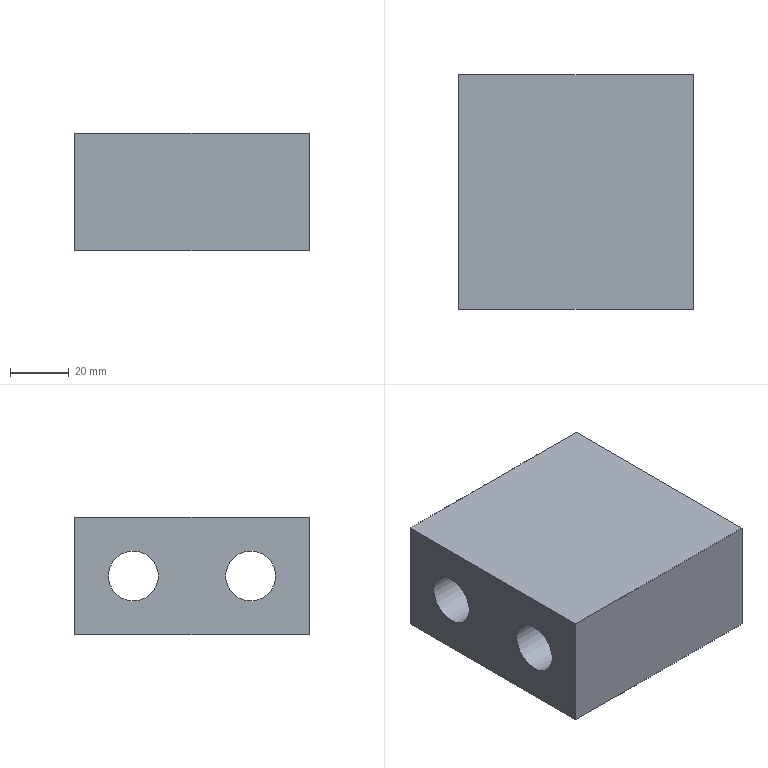Part | STEP file | 1 solid | 12 faces | box 80 x 80 x 40 mm | volume 195367 mm3 | plane 8 | cylinder 4 | commonest cylinder face diameters 17 x2 26 x2
STEP:
#1=CARTESIAN_POINT('',(350.,-102.5,-147.));
#2=VERTEX_POINT('',#1);
#3=CARTESIAN_POINT('',(350.,-102.5,-107.));
#4=VERTEX_POINT('',#3);
#5=CARTESIAN_POINT('',(350.,-102.5,-107.));
#6=DIRECTION('',(0.,0.,1.));
#7=VECTOR('',#6,1.);
#8=LINE('',#5,#7);
#9=EDGE_CURVE('',#2,#4,#8,.T.);
#10=ORIENTED_EDGE('',*,*,#9,.T.);
#11=CARTESIAN_POINT('',(430.,-102.5,-107.));
#12=VERTEX_POINT('',#11);
#13=CARTESIAN_POINT('',(350.,-102.5,-107.));
#14=DIRECTION('',(-1.,0.,0.));
#15=VECTOR('',#14,1.);
#16=LINE('',#13,#15);
#17=EDGE_CURVE('',#12,#4,#16,.T.);
#18=ORIENTED_EDGE('',*,*,#17,.F.);
#19=CARTESIAN_POINT('',(430.,-102.5,-147.));
#20=VERTEX_POINT('',#19);
#21=CARTESIAN_POINT('',(430.,-102.5,-107.));
#22=DIRECTION('',(0.,0.,1.));
#23=VECTOR('',#22,1.);
#24=LINE('',#21,#23);
#25=EDGE_CURVE('',#20,#12,#24,.T.);
#26=ORIENTED_EDGE('',*,*,#25,.F.);
#27=CARTESIAN_POINT('',(390.,-102.5,-147.));
#28=DIRECTION('',(1.,0.,0.));
#29=VECTOR('',#28,1.);
#30=LINE('',#27,#29);
#31=EDGE_CURVE('',#2,#20,#30,.T.);
#32=ORIENTED_EDGE('',*,*,#31,.F.);
#33=EDGE_LOOP('',(#10,#18,#26,#32));
#34=FACE_OUTER_BOUND('',#33,.T.);
#35=CARTESIAN_POINT('',(390.,-102.5,-127.));
#36=DIRECTION('',(0.,1.,0.));
#37=DIRECTION('',(0.,0.,1.));
#38=AXIS2_PLACEMENT_3D('',#35,#36,#37);
#39=PLANE('',#38);
#40=ADVANCED_FACE('',(#34),#39,.T.);
#41=CARTESIAN_POINT('',(350.,-182.5,-147.));
#42=VERTEX_POINT('',#41);
#43=CARTESIAN_POINT('',(430.,-182.5,-147.));
#44=VERTEX_POINT('',#43);
#45=CARTESIAN_POINT('',(350.,-182.5,-147.));
#46=DIRECTION('',(1.,0.,0.));
#47=VECTOR('',#46,1.);
#48=LINE('',#45,#47);
#49=EDGE_CURVE('',#42,#44,#48,.T.);
#50=ORIENTED_EDGE('',*,*,#49,.T.);
#51=CARTESIAN_POINT('',(430.,-182.5,-107.));
#52=VERTEX_POINT('',#51);
#53=CARTESIAN_POINT('',(430.,-182.5,-107.));
#54=DIRECTION('',(0.,0.,1.));
#55=VECTOR('',#54,1.);
#56=LINE('',#53,#55);
#57=EDGE_CURVE('',#44,#52,#56,.T.);
#58=ORIENTED_EDGE('',*,*,#57,.T.);
#59=CARTESIAN_POINT('',(350.,-182.5,-107.));
#60=VERTEX_POINT('',#59);
#61=CARTESIAN_POINT('',(350.,-182.5,-107.));
#62=DIRECTION('',(-1.,0.,0.));
#63=VECTOR('',#62,1.);
#64=LINE('',#61,#63);
#65=EDGE_CURVE('',#52,#60,#64,.T.);
#66=ORIENTED_EDGE('',*,*,#65,.T.);
#67=CARTESIAN_POINT('',(350.,-182.5,-107.));
#68=DIRECTION('',(0.,0.,1.));
#69=VECTOR('',#68,1.);
#70=LINE('',#67,#69);
#71=EDGE_CURVE('',#42,#60,#70,.T.);
#72=ORIENTED_EDGE('',*,*,#71,.F.);
#73=EDGE_LOOP('',(#50,#58,#66,#72));
#74=FACE_OUTER_BOUND('',#73,.T.);
#75=CARTESIAN_POINT('',(350.,-182.5,-107.));
#76=DIRECTION('',(0.,-1.,0.));
#77=DIRECTION('',(0.,0.,-1.));
#78=AXIS2_PLACEMENT_3D('',#75,#76,#77);
#79=PLANE('',#78);
#80=ADVANCED_FACE('',(#74),#79,.T.);
#81=CARTESIAN_POINT('',(350.,109.,-147.));
#82=DIRECTION('',(0.,-1.,0.));
#83=VECTOR('',#82,1.);
#84=LINE('',#81,#83);
#85=EDGE_CURVE('',#2,#42,#84,.T.);
#86=ORIENTED_EDGE('',*,*,#85,.F.);
#87=ORIENTED_EDGE('',*,*,#31,.T.);
#88=CARTESIAN_POINT('',(430.,109.,-147.));
#89=DIRECTION('',(0.,1.,0.));
#90=VECTOR('',#89,1.);
#91=LINE('',#88,#90);
#92=EDGE_CURVE('',#44,#20,#91,.T.);
#93=ORIENTED_EDGE('',*,*,#92,.F.);
#94=ORIENTED_EDGE('',*,*,#49,.F.);
#95=EDGE_LOOP('',(#86,#87,#93,#94));
#96=FACE_OUTER_BOUND('',#95,.T.);
#97=CARTESIAN_POINT('',(390.,110.,-147.));
#98=DIRECTION('',(0.,0.,-1.));
#99=DIRECTION('',(-1.,0.,0.));
#100=AXIS2_PLACEMENT_3D('',#97,#98,#99);
#101=PLANE('',#100);
#102=ADVANCED_FACE('',(#96),#101,.T.);
#103=ORIENTED_EDGE('',*,*,#17,.T.);
#104=CARTESIAN_POINT('',(350.,109.,-107.));
#105=DIRECTION('',(0.,-1.,0.));
#106=VECTOR('',#105,1.);
#107=LINE('',#104,#106);
#108=EDGE_CURVE('',#4,#60,#107,.T.);
#109=ORIENTED_EDGE('',*,*,#108,.T.);
#110=ORIENTED_EDGE('',*,*,#65,.F.);
#111=CARTESIAN_POINT('',(430.,109.,-107.));
#112=DIRECTION('',(0.,-1.,0.));
#113=VECTOR('',#112,1.);
#114=LINE('',#111,#113);
#115=EDGE_CURVE('',#12,#52,#114,.T.);
#116=ORIENTED_EDGE('',*,*,#115,.F.);
#117=EDGE_LOOP('',(#103,#109,#110,#116));
#118=FACE_OUTER_BOUND('',#117,.T.);
#119=CARTESIAN_POINT('',(350.,109.,-107.));
#120=DIRECTION('',(0.,0.,1.));
#121=DIRECTION('',(0.,-1.,0.));
#122=AXIS2_PLACEMENT_3D('',#119,#120,#121);
#123=PLANE('',#122);
#124=ADVANCED_FACE('',(#118),#123,.T.);
#125=CARTESIAN_POINT('',(430.,-122.5,-140.));
#126=VERTEX_POINT('',#125);
#127=CARTESIAN_POINT('',(430.,-122.5,-127.));
#128=DIRECTION('',(1.,0.,0.));
#129=DIRECTION('',(0.,0.,-1.));
#130=AXIS2_PLACEMENT_3D('',#127,#128,#129);
#131=CIRCLE('',#130,13.);
#132=EDGE_CURVE('',#126,#126,#131,.T.);
#133=ORIENTED_EDGE('',*,*,#132,.F.);
#134=EDGE_LOOP('',(#133));
#135=FACE_BOUND('',#134,.T.);
#136=CARTESIAN_POINT('',(430.,-162.5,-140.));
#137=VERTEX_POINT('',#136);
#138=CARTESIAN_POINT('',(430.,-162.5,-127.));
#139=DIRECTION('',(-1.,0.,0.));
#140=DIRECTION('',(0.,0.,-1.));
#141=AXIS2_PLACEMENT_3D('',#138,#139,#140);
#142=CIRCLE('',#141,13.);
#143=EDGE_CURVE('',#137,#137,#142,.T.);
#144=ORIENTED_EDGE('',*,*,#143,.T.);
#145=EDGE_LOOP('',(#144));
#146=FACE_BOUND('',#145,.T.);
#147=ORIENTED_EDGE('',*,*,#25,.T.);
#148=ORIENTED_EDGE('',*,*,#115,.T.);
#149=ORIENTED_EDGE('',*,*,#57,.F.);
#150=ORIENTED_EDGE('',*,*,#92,.T.);
#151=EDGE_LOOP('',(#147,#148,#149,#150));
#152=FACE_BOUND('',#151,.T.);
#153=CARTESIAN_POINT('',(430.,109.,-107.));
#154=DIRECTION('',(1.,0.,0.));
#155=DIRECTION('',(0.,-1.,0.));
#156=AXIS2_PLACEMENT_3D('',#153,#154,#155);
#157=PLANE('',#156);
#158=ADVANCED_FACE('',(#135,#146,#152),#157,.T.);
#159=CARTESIAN_POINT('',(350.,-122.5,-135.5));
#160=VERTEX_POINT('',#159);
#161=CARTESIAN_POINT('',(350.,-122.5,-127.));
#162=DIRECTION('',(-1.,0.,0.));
#163=DIRECTION('',(0.,0.,-1.));
#164=AXIS2_PLACEMENT_3D('',#161,#162,#163);
#165=CIRCLE('',#164,8.5);
#166=EDGE_CURVE('',#160,#160,#165,.T.);
#167=ORIENTED_EDGE('',*,*,#166,.F.);
#168=EDGE_LOOP('',(#167));
#169=FACE_BOUND('',#168,.T.);
#170=CARTESIAN_POINT('',(350.,-162.5,-135.5));
#171=VERTEX_POINT('',#170);
#172=CARTESIAN_POINT('',(350.,-162.5,-127.));
#173=DIRECTION('',(1.,0.,0.));
#174=DIRECTION('',(0.,0.,-1.));
#175=AXIS2_PLACEMENT_3D('',#172,#173,#174);
#176=CIRCLE('',#175,8.5);
#177=EDGE_CURVE('',#171,#171,#176,.T.);
#178=ORIENTED_EDGE('',*,*,#177,.T.);
#179=EDGE_LOOP('',(#178));
#180=FACE_BOUND('',#179,.T.);
#181=ORIENTED_EDGE('',*,*,#108,.F.);
#182=ORIENTED_EDGE('',*,*,#9,.F.);
#183=ORIENTED_EDGE('',*,*,#85,.T.);
#184=ORIENTED_EDGE('',*,*,#71,.T.);
#185=EDGE_LOOP('',(#181,#182,#183,#184));
#186=FACE_BOUND('',#185,.T.);
#187=CARTESIAN_POINT('',(350.,109.,-107.));
#188=DIRECTION('',(1.,0.,0.));
#189=DIRECTION('',(0.,-1.,0.));
#190=AXIS2_PLACEMENT_3D('',#187,#188,#189);
#191=PLANE('',#190);
#192=ADVANCED_FACE('',(#169,#180,#186),#191,.F.);
#193=CARTESIAN_POINT('',(390.,-162.5,-118.5));
#194=VERTEX_POINT('',#193);
#195=CARTESIAN_POINT('',(390.,-162.5,-127.));
#196=DIRECTION('',(-1.,0.,0.));
#197=DIRECTION('',(0.,0.,1.));
#198=AXIS2_PLACEMENT_3D('',#195,#196,#197);
#199=CIRCLE('',#198,8.5);
#200=EDGE_CURVE('',#194,#194,#199,.T.);
#201=ORIENTED_EDGE('',*,*,#200,.F.);
#202=EDGE_LOOP('',(#201));
#203=FACE_BOUND('',#202,.T.);
#204=ORIENTED_EDGE('',*,*,#177,.F.);
#205=EDGE_LOOP('',(#204));
#206=FACE_BOUND('',#205,.T.);
#207=CARTESIAN_POINT('',(350.,-162.5,-127.));
#208=DIRECTION('',(1.,0.,0.));
#209=DIRECTION('',(0.,0.,-1.));
#210=AXIS2_PLACEMENT_3D('',#207,#208,#209);
#211=CYLINDRICAL_SURFACE('',#210,8.5);
#212=ADVANCED_FACE('',(#203,#206),#211,.F.);
#213=ORIENTED_EDGE('',*,*,#200,.T.);
#214=EDGE_LOOP('',(#213));
#215=FACE_BOUND('',#214,.T.);
#216=CARTESIAN_POINT('',(390.,-162.5,-140.));
#217=VERTEX_POINT('',#216);
#218=CARTESIAN_POINT('',(390.,-162.5,-127.));
#219=DIRECTION('',(-1.,0.,0.));
#220=DIRECTION('',(0.,0.,-1.));
#221=AXIS2_PLACEMENT_3D('',#218,#219,#220);
#222=CIRCLE('',#221,13.);
#223=EDGE_CURVE('',#217,#217,#222,.T.);
#224=ORIENTED_EDGE('',*,*,#223,.F.);
#225=EDGE_LOOP('',(#224));
#226=FACE_BOUND('',#225,.T.);
#227=CARTESIAN_POINT('',(390.,-162.5,-127.));
#228=DIRECTION('',(-1.,0.,0.));
#229=DIRECTION('',(0.,0.,1.));
#230=AXIS2_PLACEMENT_3D('',#227,#228,#229);
#231=PLANE('',#230);
#232=ADVANCED_FACE('',(#215,#226),#231,.F.);
#233=ORIENTED_EDGE('',*,*,#143,.F.);
#234=EDGE_LOOP('',(#233));
#235=FACE_BOUND('',#234,.T.);
#236=ORIENTED_EDGE('',*,*,#223,.T.);
#237=EDGE_LOOP('',(#236));
#238=FACE_BOUND('',#237,.T.);
#239=CARTESIAN_POINT('',(390.,-162.5,-127.));
#240=DIRECTION('',(1.,0.,0.));
#241=DIRECTION('',(0.,0.,-1.));
#242=AXIS2_PLACEMENT_3D('',#239,#240,#241);
#243=CYLINDRICAL_SURFACE('',#242,13.);
#244=ADVANCED_FACE('',(#235,#238),#243,.F.);
#245=CARTESIAN_POINT('',(390.,-122.5,-118.5));
#246=VERTEX_POINT('',#245);
#247=CARTESIAN_POINT('',(390.,-122.5,-127.));
#248=DIRECTION('',(1.,0.,0.));
#249=DIRECTION('',(0.,0.,1.));
#250=AXIS2_PLACEMENT_3D('',#247,#248,#249);
#251=CIRCLE('',#250,8.5);
#252=EDGE_CURVE('',#246,#246,#251,.T.);
#253=ORIENTED_EDGE('',*,*,#252,.T.);
#254=EDGE_LOOP('',(#253));
#255=FACE_BOUND('',#254,.T.);
#256=ORIENTED_EDGE('',*,*,#166,.T.);
#257=EDGE_LOOP('',(#256));
#258=FACE_BOUND('',#257,.T.);
#259=CARTESIAN_POINT('',(350.,-122.5,-127.));
#260=DIRECTION('',(1.,0.,0.));
#261=DIRECTION('',(0.,0.,-1.));
#262=AXIS2_PLACEMENT_3D('',#259,#260,#261);
#263=CYLINDRICAL_SURFACE('',#262,8.5);
#264=ADVANCED_FACE('',(#255,#258),#263,.F.);
#265=ORIENTED_EDGE('',*,*,#252,.F.);
#266=EDGE_LOOP('',(#265));
#267=FACE_BOUND('',#266,.T.);
#268=CARTESIAN_POINT('',(390.,-122.5,-140.));
#269=VERTEX_POINT('',#268);
#270=CARTESIAN_POINT('',(390.,-122.5,-127.));
#271=DIRECTION('',(1.,0.,0.));
#272=DIRECTION('',(0.,0.,-1.));
#273=AXIS2_PLACEMENT_3D('',#270,#271,#272);
#274=CIRCLE('',#273,13.);
#275=EDGE_CURVE('',#269,#269,#274,.T.);
#276=ORIENTED_EDGE('',*,*,#275,.T.);
#277=EDGE_LOOP('',(#276));
#278=FACE_BOUND('',#277,.T.);
#279=CARTESIAN_POINT('',(390.,-122.5,-127.));
#280=DIRECTION('',(-1.,0.,0.));
#281=DIRECTION('',(0.,0.,1.));
#282=AXIS2_PLACEMENT_3D('',#279,#280,#281);
#283=PLANE('',#282);
#284=ADVANCED_FACE('',(#267,#278),#283,.F.);
#285=ORIENTED_EDGE('',*,*,#132,.T.);
#286=EDGE_LOOP('',(#285));
#287=FACE_BOUND('',#286,.T.);
#288=ORIENTED_EDGE('',*,*,#275,.F.);
#289=EDGE_LOOP('',(#288));
#290=FACE_BOUND('',#289,.T.);
#291=CARTESIAN_POINT('',(390.,-122.5,-127.));
#292=DIRECTION('',(1.,0.,0.));
#293=DIRECTION('',(0.,0.,-1.));
#294=AXIS2_PLACEMENT_3D('',#291,#292,#293);
#295=CYLINDRICAL_SURFACE('',#294,13.);
#296=ADVANCED_FACE('',(#287,#290),#295,.F.);
#297=CLOSED_SHELL('',(#40,#80,#102,#124,#158,#192,#212,#232,#244,#264,#284,#296));
#298=MANIFOLD_SOLID_BREP('',#297);
#299=(LENGTH_UNIT()NAMED_UNIT(*)SI_UNIT(.MILLI.,.METRE.));
#300=UNCERTAINTY_MEASURE_WITH_UNIT(LENGTH_MEASURE(0.00002),#299,'','');
#301=(NAMED_UNIT(*)PLANE_ANGLE_UNIT()SI_UNIT($,.RADIAN.));
#302=PLANE_ANGLE_MEASURE_WITH_UNIT(PLANE_ANGLE_MEASURE(0.01745),#301);
#303=DIMENSIONAL_EXPONENTS(0.,0.,0.,0.,0.,0.,0.);
#304=(CONVERSION_BASED_UNIT('DEGREE',#302)NAMED_UNIT(#303)PLANE_ANGLE_UNIT());
#305=(NAMED_UNIT(*)SI_UNIT($,.STERADIAN.)SOLID_ANGLE_UNIT());
#306=(GEOMETRIC_REPRESENTATION_CONTEXT(3)GLOBAL_UNCERTAINTY_ASSIGNED_CONTEXT((#300))GLOBAL_UNIT_ASSIGNED_CONTEXT((#299,#304,#305))REPRESENTATION_CONTEXT('',''));
#307=ADVANCED_BREP_SHAPE_REPRESENTATION('',(#298),#306);